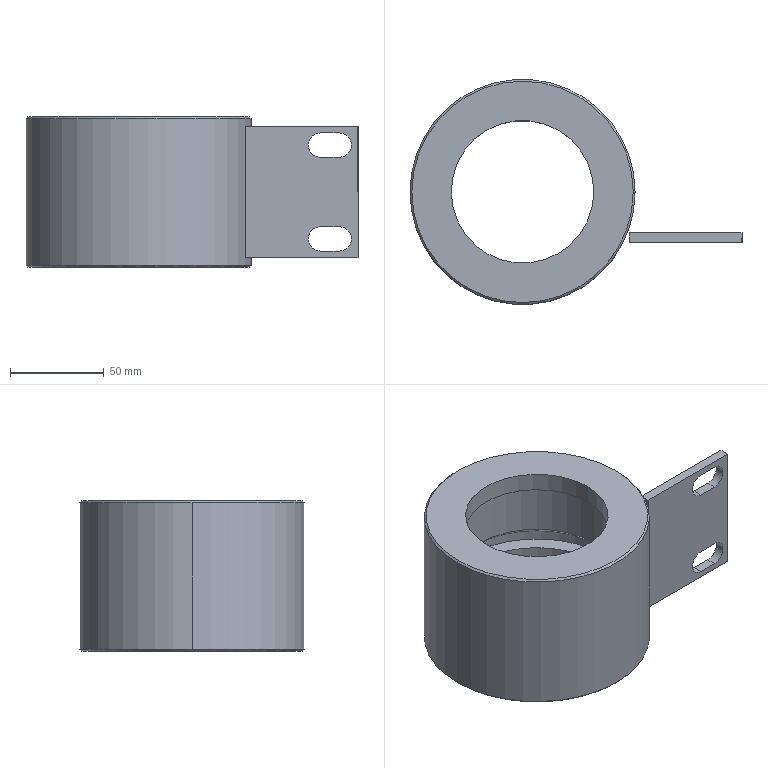Part | SolidWorks | features ICE 5, Chamfer 3, Cut 1, Extrusion 1 | 2 solids | 45 faces | box 177 x 120 x 80 mm | volume 437085 mm3 | cylinder 20 | plane 17 | cone 8 | commonest cylinder face diameters 13 x6 85 x6 76 x2 100 x2 101 x2 120 x2
STEP:
#1=CARTESIAN_POINT('',(42.5,0.,41.));
#2=VERTEX_POINT('',#1);
#3=CARTESIAN_POINT('',(-42.5,0.,41.));
#4=VERTEX_POINT('',#3);
#5=CARTESIAN_POINT('',(0.,0.,41.));
#6=DIRECTION('',(0.,0.,-1.));
#7=DIRECTION('',(-1.,0.,0.));
#8=AXIS2_PLACEMENT_3D('',#5,#6,#7);
#9=CIRCLE('',#8,42.5);
#10=EDGE_CURVE('',#2,#4,#9,.T.);
#11=ORIENTED_EDGE('',*,*,#10,.F.);
#12=CARTESIAN_POINT('',(45.5,0.,38.));
#13=VERTEX_POINT('',#12);
#14=CARTESIAN_POINT('',(42.5,0.,41.));
#15=DIRECTION('',(0.7071,0.,-0.7071));
#16=VECTOR('',#15,1000.);
#17=LINE('',#14,#16);
#18=EDGE_CURVE('',#2,#13,#17,.T.);
#19=ORIENTED_EDGE('',*,*,#18,.T.);
#20=CARTESIAN_POINT('',(-45.5,0.,38.));
#21=VERTEX_POINT('',#20);
#22=CARTESIAN_POINT('',(0.,0.,38.));
#23=DIRECTION('',(0.,0.,1.));
#24=DIRECTION('',(-1.,0.,0.));
#25=AXIS2_PLACEMENT_3D('',#22,#23,#24);
#26=CIRCLE('',#25,45.5);
#27=EDGE_CURVE('',#21,#13,#26,.T.);
#28=ORIENTED_EDGE('',*,*,#27,.F.);
#29=CARTESIAN_POINT('',(-42.5,0.,41.));
#30=DIRECTION('',(-0.7071,0.,-0.7071));
#31=VECTOR('',#30,1000.);
#32=LINE('',#29,#31);
#33=EDGE_CURVE('',#4,#21,#32,.T.);
#34=ORIENTED_EDGE('',*,*,#33,.F.);
#35=EDGE_LOOP('',(#11,#19,#28,#34));
#36=FACE_OUTER_BOUND('',#35,.T.);
#37=CARTESIAN_POINT('',(0.,0.,41.));
#38=DIRECTION('',(0.,0.,-1.));
#39=DIRECTION('',(-1.,0.,0.));
#40=AXIS2_PLACEMENT_3D('',#37,#38,#39);
#41=CONICAL_SURFACE('',#40,42.5,0.7854);
#42=ADVANCED_FACE('',(#36),#41,.F.);
#43=CARTESIAN_POINT('',(50.5,0.,38.));
#44=VERTEX_POINT('',#43);
#45=CARTESIAN_POINT('',(-50.5,0.,38.));
#46=VERTEX_POINT('',#45);
#47=CARTESIAN_POINT('',(0.,0.,38.));
#48=DIRECTION('',(0.,0.,-1.));
#49=DIRECTION('',(-1.,0.,0.));
#50=AXIS2_PLACEMENT_3D('',#47,#48,#49);
#51=CIRCLE('',#50,50.5);
#52=EDGE_CURVE('',#44,#46,#51,.T.);
#53=ORIENTED_EDGE('',*,*,#52,.F.);
#54=CARTESIAN_POINT('',(50.5,0.,29.));
#55=VERTEX_POINT('',#54);
#56=CARTESIAN_POINT('',(50.5,0.,38.));
#57=DIRECTION('',(0.,0.,-1.));
#58=VECTOR('',#57,1000.);
#59=LINE('',#56,#58);
#60=EDGE_CURVE('',#44,#55,#59,.T.);
#61=ORIENTED_EDGE('',*,*,#60,.T.);
#62=CARTESIAN_POINT('',(-50.5,0.,29.));
#63=VERTEX_POINT('',#62);
#64=CARTESIAN_POINT('',(0.,0.,29.));
#65=DIRECTION('',(0.,0.,-1.));
#66=DIRECTION('',(-1.,0.,0.));
#67=AXIS2_PLACEMENT_3D('',#64,#65,#66);
#68=CIRCLE('',#67,50.5);
#69=EDGE_CURVE('',#55,#63,#68,.T.);
#70=ORIENTED_EDGE('',*,*,#69,.T.);
#71=CARTESIAN_POINT('',(-50.5,0.,38.));
#72=DIRECTION('',(0.,0.,-1.));
#73=VECTOR('',#72,1000.);
#74=LINE('',#71,#73);
#75=EDGE_CURVE('',#46,#63,#74,.T.);
#76=ORIENTED_EDGE('',*,*,#75,.F.);
#77=EDGE_LOOP('',(#53,#61,#70,#76));
#78=FACE_OUTER_BOUND('',#77,.T.);
#79=CARTESIAN_POINT('',(0.,0.,38.));
#80=DIRECTION('',(0.,0.,-1.));
#81=DIRECTION('',(-1.,0.,0.));
#82=AXIS2_PLACEMENT_3D('',#79,#80,#81);
#83=CYLINDRICAL_SURFACE('',#82,50.5);
#84=ADVANCED_FACE('',(#78),#83,.F.);
#85=CARTESIAN_POINT('',(42.5,0.,22.));
#86=VERTEX_POINT('',#85);
#87=CARTESIAN_POINT('',(-42.5,0.,22.));
#88=VERTEX_POINT('',#87);
#89=CARTESIAN_POINT('',(0.,0.,22.));
#90=DIRECTION('',(0.,0.,-1.));
#91=DIRECTION('',(-1.,0.,0.));
#92=AXIS2_PLACEMENT_3D('',#89,#90,#91);
#93=CIRCLE('',#92,42.5);
#94=EDGE_CURVE('',#86,#88,#93,.T.);
#95=ORIENTED_EDGE('',*,*,#94,.F.);
#96=CARTESIAN_POINT('',(45.5,0.,19.));
#97=VERTEX_POINT('',#96);
#98=CARTESIAN_POINT('',(42.5,0.,22.));
#99=DIRECTION('',(0.7071,0.,-0.7071));
#100=VECTOR('',#99,1000.);
#101=LINE('',#98,#100);
#102=EDGE_CURVE('',#86,#97,#101,.T.);
#103=ORIENTED_EDGE('',*,*,#102,.T.);
#104=CARTESIAN_POINT('',(-45.5,0.,19.));
#105=VERTEX_POINT('',#104);
#106=CARTESIAN_POINT('',(0.,0.,19.));
#107=DIRECTION('',(0.,0.,1.));
#108=DIRECTION('',(-1.,0.,0.));
#109=AXIS2_PLACEMENT_3D('',#106,#107,#108);
#110=CIRCLE('',#109,45.5);
#111=EDGE_CURVE('',#105,#97,#110,.T.);
#112=ORIENTED_EDGE('',*,*,#111,.F.);
#113=CARTESIAN_POINT('',(-42.5,0.,22.));
#114=DIRECTION('',(-0.7071,0.,-0.7071));
#115=VECTOR('',#114,1000.);
#116=LINE('',#113,#115);
#117=EDGE_CURVE('',#88,#105,#116,.T.);
#118=ORIENTED_EDGE('',*,*,#117,.F.);
#119=EDGE_LOOP('',(#95,#103,#112,#118));
#120=FACE_OUTER_BOUND('',#119,.T.);
#121=CARTESIAN_POINT('',(0.,0.,22.));
#122=DIRECTION('',(0.,0.,-1.));
#123=DIRECTION('',(-1.,0.,0.));
#124=AXIS2_PLACEMENT_3D('',#121,#122,#123);
#125=CONICAL_SURFACE('',#124,42.5,0.7854);
#126=ADVANCED_FACE('',(#120),#125,.F.);
#127=CARTESIAN_POINT('',(50.,0.,19.));
#128=VERTEX_POINT('',#127);
#129=CARTESIAN_POINT('',(-50.,0.,19.));
#130=VERTEX_POINT('',#129);
#131=CARTESIAN_POINT('',(0.,0.,19.));
#132=DIRECTION('',(0.,0.,-1.));
#133=DIRECTION('',(-1.,0.,0.));
#134=AXIS2_PLACEMENT_3D('',#131,#132,#133);
#135=CIRCLE('',#134,50.);
#136=EDGE_CURVE('',#128,#130,#135,.T.);
#137=ORIENTED_EDGE('',*,*,#136,.F.);
#138=CARTESIAN_POINT('',(50.,0.,10.));
#139=VERTEX_POINT('',#138);
#140=CARTESIAN_POINT('',(50.,0.,19.));
#141=DIRECTION('',(0.,0.,-1.));
#142=VECTOR('',#141,1000.);
#143=LINE('',#140,#142);
#144=EDGE_CURVE('',#128,#139,#143,.T.);
#145=ORIENTED_EDGE('',*,*,#144,.T.);
#146=CARTESIAN_POINT('',(-50.,0.,10.));
#147=VERTEX_POINT('',#146);
#148=CARTESIAN_POINT('',(0.,0.,10.));
#149=DIRECTION('',(0.,0.,-1.));
#150=DIRECTION('',(-1.,0.,0.));
#151=AXIS2_PLACEMENT_3D('',#148,#149,#150);
#152=CIRCLE('',#151,50.);
#153=EDGE_CURVE('',#139,#147,#152,.T.);
#154=ORIENTED_EDGE('',*,*,#153,.T.);
#155=CARTESIAN_POINT('',(-50.,0.,19.));
#156=DIRECTION('',(0.,0.,-1.));
#157=VECTOR('',#156,1000.);
#158=LINE('',#155,#157);
#159=EDGE_CURVE('',#130,#147,#158,.T.);
#160=ORIENTED_EDGE('',*,*,#159,.F.);
#161=EDGE_LOOP('',(#137,#145,#154,#160));
#162=FACE_OUTER_BOUND('',#161,.T.);
#163=CARTESIAN_POINT('',(0.,0.,19.));
#164=DIRECTION('',(0.,0.,-1.));
#165=DIRECTION('',(-1.,0.,0.));
#166=AXIS2_PLACEMENT_3D('',#163,#164,#165);
#167=CYLINDRICAL_SURFACE('',#166,50.);
#168=ADVANCED_FACE('',(#162),#167,.F.);
#169=CARTESIAN_POINT('',(59.,0.,80.));
#170=VERTEX_POINT('',#169);
#171=CARTESIAN_POINT('',(-59.,0.,80.));
#172=VERTEX_POINT('',#171);
#173=CARTESIAN_POINT('',(0.,0.,80.));
#174=DIRECTION('',(0.,0.,1.));
#175=DIRECTION('',(1.,0.,0.));
#176=AXIS2_PLACEMENT_3D('',#173,#174,#175);
#177=CIRCLE('',#176,59.);
#178=EDGE_CURVE('',#170,#172,#177,.T.);
#179=ORIENTED_EDGE('',*,*,#178,.F.);
#180=CARTESIAN_POINT('',(60.,0.,79.));
#181=VERTEX_POINT('',#180);
#182=CARTESIAN_POINT('',(59.,0.,80.));
#183=DIRECTION('',(0.7071,0.,-0.7071));
#184=VECTOR('',#183,1000.);
#185=LINE('',#182,#184);
#186=EDGE_CURVE('',#170,#181,#185,.T.);
#187=ORIENTED_EDGE('',*,*,#186,.T.);
#188=CARTESIAN_POINT('',(-60.,0.,79.));
#189=VERTEX_POINT('',#188);
#190=CARTESIAN_POINT('',(0.,0.,79.));
#191=DIRECTION('',(0.,0.,-1.));
#192=DIRECTION('',(1.,0.,0.));
#193=AXIS2_PLACEMENT_3D('',#190,#191,#192);
#194=CIRCLE('',#193,60.);
#195=EDGE_CURVE('',#189,#181,#194,.T.);
#196=ORIENTED_EDGE('',*,*,#195,.F.);
#197=CARTESIAN_POINT('',(-59.,0.,80.));
#198=DIRECTION('',(-0.7071,0.,-0.7071));
#199=VECTOR('',#198,1000.);
#200=LINE('',#197,#199);
#201=EDGE_CURVE('',#172,#189,#200,.T.);
#202=ORIENTED_EDGE('',*,*,#201,.F.);
#203=EDGE_LOOP('',(#179,#187,#196,#202));
#204=FACE_OUTER_BOUND('',#203,.T.);
#205=CARTESIAN_POINT('',(0.,0.,80.));
#206=DIRECTION('',(0.,0.,-1.));
#207=DIRECTION('',(-1.,0.,0.));
#208=AXIS2_PLACEMENT_3D('',#205,#206,#207);
#209=CONICAL_SURFACE('',#208,59.,0.7854);
#210=ADVANCED_FACE('',(#204),#209,.T.);
#211=CARTESIAN_POINT('',(-59.,0.,0.));
#212=VERTEX_POINT('',#211);
#213=CARTESIAN_POINT('',(59.,0.,0.));
#214=VERTEX_POINT('',#213);
#215=CARTESIAN_POINT('',(0.,0.,0.));
#216=DIRECTION('',(0.,0.,-1.));
#217=DIRECTION('',(1.,0.,0.));
#218=AXIS2_PLACEMENT_3D('',#215,#216,#217);
#219=CIRCLE('',#218,59.);
#220=EDGE_CURVE('',#212,#214,#219,.T.);
#221=ORIENTED_EDGE('',*,*,#220,.F.);
#222=CARTESIAN_POINT('',(-60.,0.,1.));
#223=VERTEX_POINT('',#222);
#224=CARTESIAN_POINT('',(-60.,0.,1.));
#225=DIRECTION('',(-0.7071,0.,0.7071));
#226=VECTOR('',#225,1000.);
#227=LINE('',#224,#226);
#228=EDGE_CURVE('',#212,#223,#227,.T.);
#229=ORIENTED_EDGE('',*,*,#228,.T.);
#230=CARTESIAN_POINT('',(60.,0.,1.));
#231=VERTEX_POINT('',#230);
#232=CARTESIAN_POINT('',(0.,0.,1.));
#233=DIRECTION('',(0.,0.,1.));
#234=DIRECTION('',(1.,0.,0.));
#235=AXIS2_PLACEMENT_3D('',#232,#233,#234);
#236=CIRCLE('',#235,60.);
#237=EDGE_CURVE('',#231,#223,#236,.T.);
#238=ORIENTED_EDGE('',*,*,#237,.F.);
#239=CARTESIAN_POINT('',(60.,0.,1.));
#240=DIRECTION('',(0.7071,0.,0.7071));
#241=VECTOR('',#240,1000.);
#242=LINE('',#239,#241);
#243=EDGE_CURVE('',#214,#231,#242,.T.);
#244=ORIENTED_EDGE('',*,*,#243,.F.);
#245=EDGE_LOOP('',(#221,#229,#238,#244));
#246=FACE_OUTER_BOUND('',#245,.T.);
#247=CARTESIAN_POINT('',(0.,0.,1.));
#248=DIRECTION('',(0.,0.,1.));
#249=DIRECTION('',(1.,0.,0.));
#250=AXIS2_PLACEMENT_3D('',#247,#248,#249);
#251=CONICAL_SURFACE('',#250,60.,0.7854);
#252=ADVANCED_FACE('',(#246),#251,.T.);
#253=CARTESIAN_POINT('',(38.,0.,70.));
#254=VERTEX_POINT('',#253);
#255=CARTESIAN_POINT('',(-38.,0.,70.));
#256=VERTEX_POINT('',#255);
#257=CARTESIAN_POINT('',(0.,0.,70.));
#258=DIRECTION('',(0.,0.,-1.));
#259=DIRECTION('',(-1.,0.,0.));
#260=AXIS2_PLACEMENT_3D('',#257,#258,#259);
#261=CIRCLE('',#260,38.);
#262=EDGE_CURVE('',#254,#256,#261,.T.);
#263=ORIENTED_EDGE('',*,*,#262,.T.);
#264=CARTESIAN_POINT('',(-38.,0.,80.));
#265=VERTEX_POINT('',#264);
#266=CARTESIAN_POINT('',(-38.,0.,10.));
#267=DIRECTION('',(0.,0.,1.));
#268=VECTOR('',#267,1000.);
#269=LINE('',#266,#268);
#270=EDGE_CURVE('',#256,#265,#269,.T.);
#271=ORIENTED_EDGE('',*,*,#270,.T.);
#272=CARTESIAN_POINT('',(38.,0.,80.));
#273=VERTEX_POINT('',#272);
#274=CARTESIAN_POINT('',(0.,0.,80.));
#275=DIRECTION('',(0.,0.,1.));
#276=DIRECTION('',(1.,0.,0.));
#277=AXIS2_PLACEMENT_3D('',#274,#275,#276);
#278=CIRCLE('',#277,38.);
#279=EDGE_CURVE('',#265,#273,#278,.T.);
#280=ORIENTED_EDGE('',*,*,#279,.T.);
#281=CARTESIAN_POINT('',(38.,0.,10.));
#282=DIRECTION('',(0.,0.,1.));
#283=VECTOR('',#282,1000.);
#284=LINE('',#281,#283);
#285=EDGE_CURVE('',#254,#273,#284,.T.);
#286=ORIENTED_EDGE('',*,*,#285,.F.);
#287=EDGE_LOOP('',(#263,#271,#280,#286));
#288=FACE_OUTER_BOUND('',#287,.T.);
#289=CARTESIAN_POINT('',(0.,0.,10.));
#290=DIRECTION('',(0.,0.,1.));
#291=DIRECTION('',(1.,0.,0.));
#292=AXIS2_PLACEMENT_3D('',#289,#290,#291);
#293=CYLINDRICAL_SURFACE('',#292,38.);
#294=ADVANCED_FACE('',(#288),#293,.F.);
#295=CARTESIAN_POINT('',(42.5,0.,10.));
#296=VERTEX_POINT('',#295);
#297=CARTESIAN_POINT('',(-42.5,0.,10.));
#298=VERTEX_POINT('',#297);
#299=CARTESIAN_POINT('',(0.,0.,10.));
#300=DIRECTION('',(0.,0.,-1.));
#301=DIRECTION('',(-1.,0.,0.));
#302=AXIS2_PLACEMENT_3D('',#299,#300,#301);
#303=CIRCLE('',#302,42.5);
#304=EDGE_CURVE('',#296,#298,#303,.T.);
#305=ORIENTED_EDGE('',*,*,#304,.F.);
#306=CARTESIAN_POINT('',(42.5,0.,0.));
#307=VERTEX_POINT('',#306);
#308=CARTESIAN_POINT('',(42.5,0.,70.));
#309=DIRECTION('',(0.,0.,-1.));
#310=VECTOR('',#309,1000.);
#311=LINE('',#308,#310);
#312=EDGE_CURVE('',#296,#307,#311,.T.);
#313=ORIENTED_EDGE('',*,*,#312,.T.);
#314=CARTESIAN_POINT('',(-42.5,0.,0.));
#315=VERTEX_POINT('',#314);
#316=CARTESIAN_POINT('',(0.,0.,0.));
#317=DIRECTION('',(0.,0.,-1.));
#318=DIRECTION('',(-1.,0.,0.));
#319=AXIS2_PLACEMENT_3D('',#316,#317,#318);
#320=CIRCLE('',#319,42.5);
#321=EDGE_CURVE('',#307,#315,#320,.T.);
#322=ORIENTED_EDGE('',*,*,#321,.T.);
#323=CARTESIAN_POINT('',(-42.5,0.,70.));
#324=DIRECTION('',(0.,0.,-1.));
#325=VECTOR('',#324,1000.);
#326=LINE('',#323,#325);
#327=EDGE_CURVE('',#298,#315,#326,.T.);
#328=ORIENTED_EDGE('',*,*,#327,.F.);
#329=EDGE_LOOP('',(#305,#313,#322,#328));
#330=FACE_OUTER_BOUND('',#329,.T.);
#331=CARTESIAN_POINT('',(0.,0.,70.));
#332=DIRECTION('',(0.,0.,-1.));
#333=DIRECTION('',(-1.,0.,0.));
#334=AXIS2_PLACEMENT_3D('',#331,#332,#333);
#335=CYLINDRICAL_SURFACE('',#334,42.5);
#336=ADVANCED_FACE('',(#330),#335,.F.);
#337=ORIENTED_EDGE('',*,*,#195,.T.);
#338=CARTESIAN_POINT('',(60.,0.,80.));
#339=DIRECTION('',(0.,0.,-1.));
#340=VECTOR('',#339,1000.);
#341=LINE('',#338,#340);
#342=EDGE_CURVE('',#181,#231,#341,.T.);
#343=ORIENTED_EDGE('',*,*,#342,.T.);
#344=ORIENTED_EDGE('',*,*,#237,.T.);
#345=CARTESIAN_POINT('',(-60.,0.,80.));
#346=DIRECTION('',(0.,0.,-1.));
#347=VECTOR('',#346,1000.);
#348=LINE('',#345,#347);
#349=EDGE_CURVE('',#189,#223,#348,.T.);
#350=ORIENTED_EDGE('',*,*,#349,.F.);
#351=EDGE_LOOP('',(#337,#343,#344,#350));
#352=FACE_OUTER_BOUND('',#351,.T.);
#353=CARTESIAN_POINT('',(0.,0.,80.));
#354=DIRECTION('',(0.,0.,-1.));
#355=DIRECTION('',(-1.,0.,0.));
#356=AXIS2_PLACEMENT_3D('',#353,#354,#355);
#357=CYLINDRICAL_SURFACE('',#356,60.);
#358=ADVANCED_FACE('',(#352),#357,.T.);
#359=CARTESIAN_POINT('',(42.5,0.,29.));
#360=VERTEX_POINT('',#359);
#361=CARTESIAN_POINT('',(-42.5,0.,29.));
#362=VERTEX_POINT('',#361);
#363=CARTESIAN_POINT('',(0.,0.,29.));
#364=DIRECTION('',(0.,0.,-1.));
#365=DIRECTION('',(-1.,0.,0.));
#366=AXIS2_PLACEMENT_3D('',#363,#364,#365);
#367=CIRCLE('',#366,42.5);
#368=EDGE_CURVE('',#360,#362,#367,.T.);
#369=ORIENTED_EDGE('',*,*,#368,.F.);
#370=CARTESIAN_POINT('',(42.5,0.,70.));
#371=DIRECTION('',(0.,0.,-1.));
#372=VECTOR('',#371,1000.);
#373=LINE('',#370,#372);
#374=EDGE_CURVE('',#360,#86,#373,.T.);
#375=ORIENTED_EDGE('',*,*,#374,.T.);
#376=ORIENTED_EDGE('',*,*,#94,.T.);
#377=CARTESIAN_POINT('',(-42.5,0.,70.));
#378=DIRECTION('',(0.,0.,-1.));
#379=VECTOR('',#378,1000.);
#380=LINE('',#377,#379);
#381=EDGE_CURVE('',#362,#88,#380,.T.);
#382=ORIENTED_EDGE('',*,*,#381,.F.);
#383=EDGE_LOOP('',(#369,#375,#376,#382));
#384=FACE_OUTER_BOUND('',#383,.T.);
#385=CARTESIAN_POINT('',(0.,0.,70.));
#386=DIRECTION('',(0.,0.,-1.));
#387=DIRECTION('',(-1.,0.,0.));
#388=AXIS2_PLACEMENT_3D('',#385,#386,#387);
#389=CYLINDRICAL_SURFACE('',#388,42.5);
#390=ADVANCED_FACE('',(#384),#389,.F.);
#391=CARTESIAN_POINT('',(42.5,0.,70.));
#392=VERTEX_POINT('',#391);
#393=CARTESIAN_POINT('',(-42.5,0.,70.));
#394=VERTEX_POINT('',#393);
#395=CARTESIAN_POINT('',(0.,0.,70.));
#396=DIRECTION('',(0.,0.,-1.));
#397=DIRECTION('',(-1.,0.,0.));
#398=AXIS2_PLACEMENT_3D('',#395,#396,#397);
#399=CIRCLE('',#398,42.5);
#400=EDGE_CURVE('',#392,#394,#399,.T.);
#401=ORIENTED_EDGE('',*,*,#400,.F.);
#402=CARTESIAN_POINT('',(42.5,0.,70.));
#403=DIRECTION('',(0.,0.,-1.));
#404=VECTOR('',#403,1000.);
#405=LINE('',#402,#404);
#406=EDGE_CURVE('',#392,#2,#405,.T.);
#407=ORIENTED_EDGE('',*,*,#406,.T.);
#408=ORIENTED_EDGE('',*,*,#10,.T.);
#409=CARTESIAN_POINT('',(-42.5,0.,70.));
#410=DIRECTION('',(0.,0.,-1.));
#411=VECTOR('',#410,1000.);
#412=LINE('',#409,#411);
#413=EDGE_CURVE('',#394,#4,#412,.T.);
#414=ORIENTED_EDGE('',*,*,#413,.F.);
#415=EDGE_LOOP('',(#401,#407,#408,#414));
#416=FACE_OUTER_BOUND('',#415,.T.);
#417=CARTESIAN_POINT('',(0.,0.,70.));
#418=DIRECTION('',(0.,0.,-1.));
#419=DIRECTION('',(-1.,0.,0.));
#420=AXIS2_PLACEMENT_3D('',#417,#418,#419);
#421=CYLINDRICAL_SURFACE('',#420,42.5);
#422=ADVANCED_FACE('',(#416),#421,.F.);
#423=ORIENTED_EDGE('',*,*,#406,.F.);
#424=CARTESIAN_POINT('',(0.,0.,70.));
#425=DIRECTION('',(0.,0.,-1.));
#426=DIRECTION('',(-1.,0.,0.));
#427=AXIS2_PLACEMENT_3D('',#424,#425,#426);
#428=CIRCLE('',#427,42.5);
#429=EDGE_CURVE('',#394,#392,#428,.T.);
#430=ORIENTED_EDGE('',*,*,#429,.F.);
#431=ORIENTED_EDGE('',*,*,#413,.T.);
#432=CARTESIAN_POINT('',(0.,0.,41.));
#433=DIRECTION('',(0.,0.,-1.));
#434=DIRECTION('',(-1.,0.,0.));
#435=AXIS2_PLACEMENT_3D('',#432,#433,#434);
#436=CIRCLE('',#435,42.5);
#437=EDGE_CURVE('',#4,#2,#436,.T.);
#438=ORIENTED_EDGE('',*,*,#437,.T.);
#439=EDGE_LOOP('',(#423,#430,#431,#438));
#440=FACE_OUTER_BOUND('',#439,.T.);
#441=CARTESIAN_POINT('',(0.,0.,70.));
#442=DIRECTION('',(0.,0.,-1.));
#443=DIRECTION('',(-1.,0.,0.));
#444=AXIS2_PLACEMENT_3D('',#441,#442,#443);
#445=CYLINDRICAL_SURFACE('',#444,42.5);
#446=ADVANCED_FACE('',(#440),#445,.F.);
#447=ORIENTED_EDGE('',*,*,#374,.F.);
#448=CARTESIAN_POINT('',(0.,0.,29.));
#449=DIRECTION('',(0.,0.,-1.));
#450=DIRECTION('',(-1.,0.,0.));
#451=AXIS2_PLACEMENT_3D('',#448,#449,#450);
#452=CIRCLE('',#451,42.5);
#453=EDGE_CURVE('',#362,#360,#452,.T.);
#454=ORIENTED_EDGE('',*,*,#453,.F.);
#455=ORIENTED_EDGE('',*,*,#381,.T.);
#456=CARTESIAN_POINT('',(0.,0.,22.));
#457=DIRECTION('',(0.,0.,-1.));
#458=DIRECTION('',(-1.,0.,0.));
#459=AXIS2_PLACEMENT_3D('',#456,#457,#458);
#460=CIRCLE('',#459,42.5);
#461=EDGE_CURVE('',#88,#86,#460,.T.);
#462=ORIENTED_EDGE('',*,*,#461,.T.);
#463=EDGE_LOOP('',(#447,#454,#455,#462));
#464=FACE_OUTER_BOUND('',#463,.T.);
#465=CARTESIAN_POINT('',(0.,0.,70.));
#466=DIRECTION('',(0.,0.,-1.));
#467=DIRECTION('',(-1.,0.,0.));
#468=AXIS2_PLACEMENT_3D('',#465,#466,#467);
#469=CYLINDRICAL_SURFACE('',#468,42.5);
#470=ADVANCED_FACE('',(#464),#469,.F.);
#471=ORIENTED_EDGE('',*,*,#342,.F.);
#472=CARTESIAN_POINT('',(0.,0.,79.));
#473=DIRECTION('',(0.,0.,-1.));
#474=DIRECTION('',(1.,0.,0.));
#475=AXIS2_PLACEMENT_3D('',#472,#473,#474);
#476=CIRCLE('',#475,60.);
#477=EDGE_CURVE('',#181,#189,#476,.T.);
#478=ORIENTED_EDGE('',*,*,#477,.T.);
#479=ORIENTED_EDGE('',*,*,#349,.T.);
#480=CARTESIAN_POINT('',(0.,0.,1.));
#481=DIRECTION('',(0.,0.,1.));
#482=DIRECTION('',(1.,0.,0.));
#483=AXIS2_PLACEMENT_3D('',#480,#481,#482);
#484=CIRCLE('',#483,60.);
#485=EDGE_CURVE('',#223,#231,#484,.T.);
#486=ORIENTED_EDGE('',*,*,#485,.T.);
#487=EDGE_LOOP('',(#471,#478,#479,#486));
#488=FACE_OUTER_BOUND('',#487,.T.);
#489=CARTESIAN_POINT('',(0.,0.,80.));
#490=DIRECTION('',(0.,0.,-1.));
#491=DIRECTION('',(-1.,0.,0.));
#492=AXIS2_PLACEMENT_3D('',#489,#490,#491);
#493=CYLINDRICAL_SURFACE('',#492,60.);
#494=ADVANCED_FACE('',(#488),#493,.T.);
#495=CARTESIAN_POINT('',(0.,0.,80.));
#496=DIRECTION('',(0.,0.,1.));
#497=DIRECTION('',(1.,0.,0.));
#498=AXIS2_PLACEMENT_3D('',#495,#496,#497);
#499=CIRCLE('',#498,59.);
#500=EDGE_CURVE('',#172,#170,#499,.T.);
#501=ORIENTED_EDGE('',*,*,#500,.T.);
#502=ORIENTED_EDGE('',*,*,#178,.T.);
#503=EDGE_LOOP('',(#501,#502));
#504=FACE_OUTER_BOUND('',#503,.T.);
#505=CARTESIAN_POINT('',(0.,0.,80.));
#506=DIRECTION('',(0.,0.,1.));
#507=DIRECTION('',(1.,0.,0.));
#508=AXIS2_PLACEMENT_3D('',#505,#506,#507);
#509=CIRCLE('',#508,38.);
#510=EDGE_CURVE('',#273,#265,#509,.T.);
#511=ORIENTED_EDGE('',*,*,#510,.F.);
#512=ORIENTED_EDGE('',*,*,#279,.F.);
#513=EDGE_LOOP('',(#511,#512));
#514=FACE_BOUND('',#513,.T.);
#515=CARTESIAN_POINT('',(0.,0.,80.));
#516=DIRECTION('',(0.,0.,1.));
#517=DIRECTION('',(1.,0.,0.));
#518=AXIS2_PLACEMENT_3D('',#515,#516,#517);
#519=PLANE('',#518);
#520=ADVANCED_FACE('',(#504,#514),#519,.T.);
#521=CARTESIAN_POINT('',(0.,0.,0.));
#522=DIRECTION('',(0.,0.,-1.));
#523=DIRECTION('',(1.,0.,0.));
#524=AXIS2_PLACEMENT_3D('',#521,#522,#523);
#525=CIRCLE('',#524,59.);
#526=EDGE_CURVE('',#214,#212,#525,.T.);
#527=ORIENTED_EDGE('',*,*,#526,.T.);
#528=ORIENTED_EDGE('',*,*,#220,.T.);
#529=EDGE_LOOP('',(#527,#528));
#530=FACE_OUTER_BOUND('',#529,.T.);
#531=CARTESIAN_POINT('',(0.,0.,0.));
#532=DIRECTION('',(0.,0.,-1.));
#533=DIRECTION('',(-1.,0.,0.));
#534=AXIS2_PLACEMENT_3D('',#531,#532,#533);
#535=CIRCLE('',#534,42.5);
#536=EDGE_CURVE('',#315,#307,#535,.T.);
#537=ORIENTED_EDGE('',*,*,#536,.F.);
#538=ORIENTED_EDGE('',*,*,#321,.F.);
#539=EDGE_LOOP('',(#537,#538));
#540=FACE_BOUND('',#539,.T.);
#541=CARTESIAN_POINT('',(0.,0.,0.));
#542=DIRECTION('',(0.,0.,1.));
#543=DIRECTION('',(1.,0.,0.));
#544=AXIS2_PLACEMENT_3D('',#541,#542,#543);
#545=PLANE('',#544);
#546=ADVANCED_FACE('',(#530,#540),#545,.F.);
#547=ORIENTED_EDGE('',*,*,#312,.F.);
#548=CARTESIAN_POINT('',(0.,0.,10.));
#549=DIRECTION('',(0.,0.,-1.));
#550=DIRECTION('',(-1.,0.,0.));
#551=AXIS2_PLACEMENT_3D('',#548,#549,#550);
#552=CIRCLE('',#551,42.5);
#553=EDGE_CURVE('',#298,#296,#552,.T.);
#554=ORIENTED_EDGE('',*,*,#553,.F.);
#555=ORIENTED_EDGE('',*,*,#327,.T.);
#556=ORIENTED_EDGE('',*,*,#536,.T.);
#557=EDGE_LOOP('',(#547,#554,#555,#556));
#558=FACE_OUTER_BOUND('',#557,.T.);
#559=CARTESIAN_POINT('',(0.,0.,70.));
#560=DIRECTION('',(0.,0.,-1.));
#561=DIRECTION('',(-1.,0.,0.));
#562=AXIS2_PLACEMENT_3D('',#559,#560,#561);
#563=CYLINDRICAL_SURFACE('',#562,42.5);
#564=ADVANCED_FACE('',(#558),#563,.F.);
#565=ORIENTED_EDGE('',*,*,#262,.F.);
#566=CARTESIAN_POINT('',(0.,0.,70.));
#567=DIRECTION('',(0.,0.,-1.));
#568=DIRECTION('',(-1.,0.,0.));
#569=AXIS2_PLACEMENT_3D('',#566,#567,#568);
#570=CIRCLE('',#569,38.);
#571=EDGE_CURVE('',#256,#254,#570,.T.);
#572=ORIENTED_EDGE('',*,*,#571,.F.);
#573=EDGE_LOOP('',(#565,#572));
#574=FACE_BOUND('',#573,.T.);
#575=ORIENTED_EDGE('',*,*,#429,.T.);
#576=ORIENTED_EDGE('',*,*,#400,.T.);
#577=EDGE_LOOP('',(#575,#576));
#578=FACE_OUTER_BOUND('',#577,.T.);
#579=CARTESIAN_POINT('',(0.,0.,70.));
#580=DIRECTION('',(0.,0.,-1.));
#581=DIRECTION('',(-1.,0.,0.));
#582=AXIS2_PLACEMENT_3D('',#579,#580,#581);
#583=PLANE('',#582);
#584=ADVANCED_FACE('',(#574,#578),#583,.T.);
#585=ORIENTED_EDGE('',*,*,#270,.F.);
#586=ORIENTED_EDGE('',*,*,#571,.T.);
#587=ORIENTED_EDGE('',*,*,#285,.T.);
#588=ORIENTED_EDGE('',*,*,#510,.T.);
#589=EDGE_LOOP('',(#585,#586,#587,#588));
#590=FACE_OUTER_BOUND('',#589,.T.);
#591=CARTESIAN_POINT('',(0.,0.,10.));
#592=DIRECTION('',(0.,0.,1.));
#593=DIRECTION('',(1.,0.,0.));
#594=AXIS2_PLACEMENT_3D('',#591,#592,#593);
#595=CYLINDRICAL_SURFACE('',#594,38.);
#596=ADVANCED_FACE('',(#590),#595,.F.);
#597=ORIENTED_EDGE('',*,*,#228,.F.);
#598=ORIENTED_EDGE('',*,*,#526,.F.);
#599=ORIENTED_EDGE('',*,*,#243,.T.);
#600=ORIENTED_EDGE('',*,*,#485,.F.);
#601=EDGE_LOOP('',(#597,#598,#599,#600));
#602=FACE_OUTER_BOUND('',#601,.T.);
#603=CARTESIAN_POINT('',(0.,0.,1.));
#604=DIRECTION('',(0.,0.,1.));
#605=DIRECTION('',(1.,0.,0.));
#606=AXIS2_PLACEMENT_3D('',#603,#604,#605);
#607=CONICAL_SURFACE('',#606,60.,0.7854);
#608=ADVANCED_FACE('',(#602),#607,.T.);
#609=ORIENTED_EDGE('',*,*,#186,.F.);
#610=ORIENTED_EDGE('',*,*,#500,.F.);
#611=ORIENTED_EDGE('',*,*,#201,.T.);
#612=ORIENTED_EDGE('',*,*,#477,.F.);
#613=EDGE_LOOP('',(#609,#610,#611,#612));
#614=FACE_OUTER_BOUND('',#613,.T.);
#615=CARTESIAN_POINT('',(0.,0.,80.));
#616=DIRECTION('',(0.,0.,-1.));
#617=DIRECTION('',(-1.,0.,0.));
#618=AXIS2_PLACEMENT_3D('',#615,#616,#617);
#619=CONICAL_SURFACE('',#618,59.,0.7854);
#620=ADVANCED_FACE('',(#614),#619,.T.);
#621=ORIENTED_EDGE('',*,*,#144,.F.);
#622=CARTESIAN_POINT('',(0.,0.,19.));
#623=DIRECTION('',(0.,0.,-1.));
#624=DIRECTION('',(-1.,0.,0.));
#625=AXIS2_PLACEMENT_3D('',#622,#623,#624);
#626=CIRCLE('',#625,50.);
#627=EDGE_CURVE('',#130,#128,#626,.T.);
#628=ORIENTED_EDGE('',*,*,#627,.F.);
#629=ORIENTED_EDGE('',*,*,#159,.T.);
#630=CARTESIAN_POINT('',(0.,0.,10.));
#631=DIRECTION('',(0.,0.,-1.));
#632=DIRECTION('',(-1.,0.,0.));
#633=AXIS2_PLACEMENT_3D('',#630,#631,#632);
#634=CIRCLE('',#633,50.);
#635=EDGE_CURVE('',#147,#139,#634,.T.);
#636=ORIENTED_EDGE('',*,*,#635,.T.);
#637=EDGE_LOOP('',(#621,#628,#629,#636));
#638=FACE_OUTER_BOUND('',#637,.T.);
#639=CARTESIAN_POINT('',(0.,0.,19.));
#640=DIRECTION('',(0.,0.,-1.));
#641=DIRECTION('',(-1.,0.,0.));
#642=AXIS2_PLACEMENT_3D('',#639,#640,#641);
#643=CYLINDRICAL_SURFACE('',#642,50.);
#644=ADVANCED_FACE('',(#638),#643,.F.);
#645=ORIENTED_EDGE('',*,*,#111,.T.);
#646=CARTESIAN_POINT('',(0.,0.,19.));
#647=DIRECTION('',(0.,0.,1.));
#648=DIRECTION('',(-1.,0.,0.));
#649=AXIS2_PLACEMENT_3D('',#646,#647,#648);
#650=CIRCLE('',#649,45.5);
#651=EDGE_CURVE('',#97,#105,#650,.T.);
#652=ORIENTED_EDGE('',*,*,#651,.T.);
#653=EDGE_LOOP('',(#645,#652));
#654=FACE_BOUND('',#653,.T.);
#655=ORIENTED_EDGE('',*,*,#627,.T.);
#656=ORIENTED_EDGE('',*,*,#136,.T.);
#657=EDGE_LOOP('',(#655,#656));
#658=FACE_OUTER_BOUND('',#657,.T.);
#659=CARTESIAN_POINT('',(0.,0.,19.));
#660=DIRECTION('',(0.,0.,-1.));
#661=DIRECTION('',(-1.,0.,0.));
#662=AXIS2_PLACEMENT_3D('',#659,#660,#661);
#663=PLANE('',#662);
#664=ADVANCED_FACE('',(#654,#658),#663,.T.);
#665=ORIENTED_EDGE('',*,*,#553,.T.);
#666=ORIENTED_EDGE('',*,*,#304,.T.);
#667=EDGE_LOOP('',(#665,#666));
#668=FACE_BOUND('',#667,.T.);
#669=ORIENTED_EDGE('',*,*,#635,.F.);
#670=ORIENTED_EDGE('',*,*,#153,.F.);
#671=EDGE_LOOP('',(#669,#670));
#672=FACE_OUTER_BOUND('',#671,.T.);
#673=CARTESIAN_POINT('',(0.,0.,10.));
#674=DIRECTION('',(0.,0.,-1.));
#675=DIRECTION('',(-1.,0.,0.));
#676=AXIS2_PLACEMENT_3D('',#673,#674,#675);
#677=PLANE('',#676);
#678=ADVANCED_FACE('',(#668,#672),#677,.F.);
#679=ORIENTED_EDGE('',*,*,#102,.F.);
#680=ORIENTED_EDGE('',*,*,#461,.F.);
#681=ORIENTED_EDGE('',*,*,#117,.T.);
#682=ORIENTED_EDGE('',*,*,#651,.F.);
#683=EDGE_LOOP('',(#679,#680,#681,#682));
#684=FACE_OUTER_BOUND('',#683,.T.);
#685=CARTESIAN_POINT('',(0.,0.,22.));
#686=DIRECTION('',(0.,0.,-1.));
#687=DIRECTION('',(-1.,0.,0.));
#688=AXIS2_PLACEMENT_3D('',#685,#686,#687);
#689=CONICAL_SURFACE('',#688,42.5,0.7854);
#690=ADVANCED_FACE('',(#684),#689,.F.);
#691=ORIENTED_EDGE('',*,*,#60,.F.);
#692=CARTESIAN_POINT('',(0.,0.,38.));
#693=DIRECTION('',(0.,0.,-1.));
#694=DIRECTION('',(-1.,0.,0.));
#695=AXIS2_PLACEMENT_3D('',#692,#693,#694);
#696=CIRCLE('',#695,50.5);
#697=EDGE_CURVE('',#46,#44,#696,.T.);
#698=ORIENTED_EDGE('',*,*,#697,.F.);
#699=ORIENTED_EDGE('',*,*,#75,.T.);
#700=CARTESIAN_POINT('',(0.,0.,29.));
#701=DIRECTION('',(0.,0.,-1.));
#702=DIRECTION('',(-1.,0.,0.));
#703=AXIS2_PLACEMENT_3D('',#700,#701,#702);
#704=CIRCLE('',#703,50.5);
#705=EDGE_CURVE('',#63,#55,#704,.T.);
#706=ORIENTED_EDGE('',*,*,#705,.T.);
#707=EDGE_LOOP('',(#691,#698,#699,#706));
#708=FACE_OUTER_BOUND('',#707,.T.);
#709=CARTESIAN_POINT('',(0.,0.,38.));
#710=DIRECTION('',(0.,0.,-1.));
#711=DIRECTION('',(-1.,0.,0.));
#712=AXIS2_PLACEMENT_3D('',#709,#710,#711);
#713=CYLINDRICAL_SURFACE('',#712,50.5);
#714=ADVANCED_FACE('',(#708),#713,.F.);
#715=ORIENTED_EDGE('',*,*,#27,.T.);
#716=CARTESIAN_POINT('',(0.,0.,38.));
#717=DIRECTION('',(0.,0.,1.));
#718=DIRECTION('',(-1.,0.,0.));
#719=AXIS2_PLACEMENT_3D('',#716,#717,#718);
#720=CIRCLE('',#719,45.5);
#721=EDGE_CURVE('',#13,#21,#720,.T.);
#722=ORIENTED_EDGE('',*,*,#721,.T.);
#723=EDGE_LOOP('',(#715,#722));
#724=FACE_BOUND('',#723,.T.);
#725=ORIENTED_EDGE('',*,*,#697,.T.);
#726=ORIENTED_EDGE('',*,*,#52,.T.);
#727=EDGE_LOOP('',(#725,#726));
#728=FACE_OUTER_BOUND('',#727,.T.);
#729=CARTESIAN_POINT('',(0.,0.,38.));
#730=DIRECTION('',(0.,0.,-1.));
#731=DIRECTION('',(-1.,0.,0.));
#732=AXIS2_PLACEMENT_3D('',#729,#730,#731);
#733=PLANE('',#732);
#734=ADVANCED_FACE('',(#724,#728),#733,.T.);
#735=ORIENTED_EDGE('',*,*,#453,.T.);
#736=ORIENTED_EDGE('',*,*,#368,.T.);
#737=EDGE_LOOP('',(#735,#736));
#738=FACE_BOUND('',#737,.T.);
#739=ORIENTED_EDGE('',*,*,#705,.F.);
#740=ORIENTED_EDGE('',*,*,#69,.F.);
#741=EDGE_LOOP('',(#739,#740));
#742=FACE_OUTER_BOUND('',#741,.T.);
#743=CARTESIAN_POINT('',(0.,0.,29.));
#744=DIRECTION('',(0.,0.,-1.));
#745=DIRECTION('',(-1.,0.,0.));
#746=AXIS2_PLACEMENT_3D('',#743,#744,#745);
#747=PLANE('',#746);
#748=ADVANCED_FACE('',(#738,#742),#747,.F.);
#749=ORIENTED_EDGE('',*,*,#18,.F.);
#750=ORIENTED_EDGE('',*,*,#437,.F.);
#751=ORIENTED_EDGE('',*,*,#33,.T.);
#752=ORIENTED_EDGE('',*,*,#721,.F.);
#753=EDGE_LOOP('',(#749,#750,#751,#752));
#754=FACE_OUTER_BOUND('',#753,.T.);
#755=CARTESIAN_POINT('',(0.,0.,41.));
#756=DIRECTION('',(0.,0.,-1.));
#757=DIRECTION('',(-1.,0.,0.));
#758=AXIS2_PLACEMENT_3D('',#755,#756,#757);
#759=CONICAL_SURFACE('',#758,42.5,0.7854);
#760=ADVANCED_FACE('',(#754),#759,.F.);
#761=CLOSED_SHELL('',(#42,#84,#126,#168,#210,#252,#294,#336,#358,#390,#422,#446,#470,#494,#520,#546,#564,#584,#596,#608,#620,#644,#664,#678,#690,#714,#734,#748,#760));
#762=MANIFOLD_SOLID_BREP('',#761);
#763=CARTESIAN_POINT('',(113.5,-21.831,15.));
#764=VERTEX_POINT('',#763);
#765=CARTESIAN_POINT('',(107.,-21.831,21.5));
#766=VERTEX_POINT('',#765);
#767=CARTESIAN_POINT('',(107.,-21.831,15.));
#768=DIRECTION('',(0.,-1.,0.));
#769=DIRECTION('',(1.,0.,0.));
#770=AXIS2_PLACEMENT_3D('',#767,#768,#769);
#771=CIRCLE('',#770,6.5);
#772=EDGE_CURVE('',#764,#766,#771,.T.);
#773=ORIENTED_EDGE('',*,*,#772,.F.);
#774=CARTESIAN_POINT('',(113.5,-26.831,15.));
#775=VERTEX_POINT('',#774);
#776=CARTESIAN_POINT('',(113.5,-21.831,15.));
#777=DIRECTION('',(0.,-1.,0.));
#778=VECTOR('',#777,1000.);
#779=LINE('',#776,#778);
#780=EDGE_CURVE('',#764,#775,#779,.T.);
#781=ORIENTED_EDGE('',*,*,#780,.T.);
#782=CARTESIAN_POINT('',(107.,-26.831,21.5));
#783=VERTEX_POINT('',#782);
#784=CARTESIAN_POINT('',(107.,-26.831,15.));
#785=DIRECTION('',(0.,-1.,0.));
#786=DIRECTION('',(1.,0.,0.));
#787=AXIS2_PLACEMENT_3D('',#784,#785,#786);
#788=CIRCLE('',#787,6.5);
#789=EDGE_CURVE('',#775,#783,#788,.T.);
#790=ORIENTED_EDGE('',*,*,#789,.T.);
#791=CARTESIAN_POINT('',(107.,-21.831,21.5));
#792=DIRECTION('',(0.,-1.,0.));
#793=VECTOR('',#792,1000.);
#794=LINE('',#791,#793);
#795=EDGE_CURVE('',#766,#783,#794,.T.);
#796=ORIENTED_EDGE('',*,*,#795,.F.);
#797=EDGE_LOOP('',(#773,#781,#790,#796));
#798=FACE_OUTER_BOUND('',#797,.T.);
#799=CARTESIAN_POINT('',(107.,-21.831,15.));
#800=DIRECTION('',(0.,-1.,0.));
#801=DIRECTION('',(1.,0.,0.));
#802=AXIS2_PLACEMENT_3D('',#799,#800,#801);
#803=CYLINDRICAL_SURFACE('',#802,6.5);
#804=ADVANCED_FACE('',(#798),#803,.F.);
#805=CARTESIAN_POINT('',(113.5,-21.831,65.));
#806=VERTEX_POINT('',#805);
#807=CARTESIAN_POINT('',(107.,-21.831,71.5));
#808=VERTEX_POINT('',#807);
#809=CARTESIAN_POINT('',(107.,-21.831,65.));
#810=DIRECTION('',(0.,-1.,0.));
#811=DIRECTION('',(-1.,0.,0.));
#812=AXIS2_PLACEMENT_3D('',#809,#810,#811);
#813=CIRCLE('',#812,6.5);
#814=EDGE_CURVE('',#806,#808,#813,.T.);
#815=ORIENTED_EDGE('',*,*,#814,.F.);
#816=CARTESIAN_POINT('',(113.5,-26.831,65.));
#817=VERTEX_POINT('',#816);
#818=CARTESIAN_POINT('',(113.5,-21.831,65.));
#819=DIRECTION('',(0.,-1.,0.));
#820=VECTOR('',#819,1000.);
#821=LINE('',#818,#820);
#822=EDGE_CURVE('',#806,#817,#821,.T.);
#823=ORIENTED_EDGE('',*,*,#822,.T.);
#824=CARTESIAN_POINT('',(107.,-26.831,71.5));
#825=VERTEX_POINT('',#824);
#826=CARTESIAN_POINT('',(107.,-26.831,65.));
#827=DIRECTION('',(0.,-1.,0.));
#828=DIRECTION('',(-1.,0.,0.));
#829=AXIS2_PLACEMENT_3D('',#826,#827,#828);
#830=CIRCLE('',#829,6.5);
#831=EDGE_CURVE('',#817,#825,#830,.T.);
#832=ORIENTED_EDGE('',*,*,#831,.T.);
#833=CARTESIAN_POINT('',(107.,-21.831,71.5));
#834=DIRECTION('',(0.,-1.,0.));
#835=VECTOR('',#834,1000.);
#836=LINE('',#833,#835);
#837=EDGE_CURVE('',#808,#825,#836,.T.);
#838=ORIENTED_EDGE('',*,*,#837,.F.);
#839=EDGE_LOOP('',(#815,#823,#832,#838));
#840=FACE_OUTER_BOUND('',#839,.T.);
#841=CARTESIAN_POINT('',(107.,-21.831,65.));
#842=DIRECTION('',(0.,-1.,0.));
#843=DIRECTION('',(1.,0.,0.));
#844=AXIS2_PLACEMENT_3D('',#841,#842,#843);
#845=CYLINDRICAL_SURFACE('',#844,6.5);
#846=ADVANCED_FACE('',(#840),#845,.F.);
#847=CARTESIAN_POINT('',(117.,-26.831,75.));
#848=VERTEX_POINT('',#847);
#849=CARTESIAN_POINT('',(117.,-21.831,75.));
#850=VERTEX_POINT('',#849);
#851=CARTESIAN_POINT('',(117.,-21.831,75.));
#852=DIRECTION('',(0.,1.,0.));
#853=VECTOR('',#852,1000.);
#854=LINE('',#851,#853);
#855=EDGE_CURVE('',#848,#850,#854,.T.);
#856=ORIENTED_EDGE('',*,*,#855,.T.);
#857=CARTESIAN_POINT('',(57.,-21.831,75.));
#858=VERTEX_POINT('',#857);
#859=CARTESIAN_POINT('',(57.,-21.831,75.));
#860=DIRECTION('',(1.,0.,0.));
#861=VECTOR('',#860,1000.);
#862=LINE('',#859,#861);
#863=EDGE_CURVE('',#858,#850,#862,.T.);
#864=ORIENTED_EDGE('',*,*,#863,.F.);
#865=CARTESIAN_POINT('',(57.,-26.831,75.));
#866=VERTEX_POINT('',#865);
#867=CARTESIAN_POINT('',(57.,-21.831,75.));
#868=DIRECTION('',(0.,1.,0.));
#869=VECTOR('',#868,1000.);
#870=LINE('',#867,#869);
#871=EDGE_CURVE('',#866,#858,#870,.T.);
#872=ORIENTED_EDGE('',*,*,#871,.F.);
#873=CARTESIAN_POINT('',(57.,-26.831,75.));
#874=DIRECTION('',(1.,0.,0.));
#875=VECTOR('',#874,1000.);
#876=LINE('',#873,#875);
#877=EDGE_CURVE('',#866,#848,#876,.T.);
#878=ORIENTED_EDGE('',*,*,#877,.T.);
#879=EDGE_LOOP('',(#856,#864,#872,#878));
#880=FACE_OUTER_BOUND('',#879,.T.);
#881=CARTESIAN_POINT('',(57.,-21.831,75.));
#882=DIRECTION('',(0.,0.,-1.));
#883=DIRECTION('',(-1.,0.,0.));
#884=AXIS2_PLACEMENT_3D('',#881,#882,#883);
#885=PLANE('',#884);
#886=ADVANCED_FACE('',(#880),#885,.F.);
#887=CARTESIAN_POINT('',(97.,-21.831,21.5));
#888=VERTEX_POINT('',#887);
#889=CARTESIAN_POINT('',(97.,-21.831,21.5));
#890=DIRECTION('',(-1.,0.,0.));
#891=VECTOR('',#890,1000.);
#892=LINE('',#889,#891);
#893=EDGE_CURVE('',#766,#888,#892,.T.);
#894=ORIENTED_EDGE('',*,*,#893,.T.);
#895=CARTESIAN_POINT('',(97.,-21.831,8.5));
#896=VERTEX_POINT('',#895);
#897=CARTESIAN_POINT('',(97.,-21.831,15.));
#898=DIRECTION('',(0.,-1.,0.));
#899=DIRECTION('',(-1.,0.,0.));
#900=AXIS2_PLACEMENT_3D('',#897,#898,#899);
#901=CIRCLE('',#900,6.5);
#902=EDGE_CURVE('',#888,#896,#901,.T.);
#903=ORIENTED_EDGE('',*,*,#902,.T.);
#904=CARTESIAN_POINT('',(107.,-21.831,8.5));
#905=VERTEX_POINT('',#904);
#906=CARTESIAN_POINT('',(97.,-21.831,8.5));
#907=DIRECTION('',(1.,0.,0.));
#908=VECTOR('',#907,1000.);
#909=LINE('',#906,#908);
#910=EDGE_CURVE('',#896,#905,#909,.T.);
#911=ORIENTED_EDGE('',*,*,#910,.T.);
#912=CARTESIAN_POINT('',(107.,-21.831,15.));
#913=DIRECTION('',(0.,-1.,0.));
#914=DIRECTION('',(1.,0.,0.));
#915=AXIS2_PLACEMENT_3D('',#912,#913,#914);
#916=CIRCLE('',#915,6.5);
#917=EDGE_CURVE('',#905,#764,#916,.T.);
#918=ORIENTED_EDGE('',*,*,#917,.T.);
#919=ORIENTED_EDGE('',*,*,#772,.T.);
#920=EDGE_LOOP('',(#894,#903,#911,#918,#919));
#921=FACE_BOUND('',#920,.T.);
#922=CARTESIAN_POINT('',(97.,-21.831,58.5));
#923=VERTEX_POINT('',#922);
#924=CARTESIAN_POINT('',(107.,-21.831,58.5));
#925=VERTEX_POINT('',#924);
#926=CARTESIAN_POINT('',(97.,-21.831,58.5));
#927=DIRECTION('',(1.,0.,0.));
#928=VECTOR('',#927,1000.);
#929=LINE('',#926,#928);
#930=EDGE_CURVE('',#923,#925,#929,.T.);
#931=ORIENTED_EDGE('',*,*,#930,.T.);
#932=CARTESIAN_POINT('',(107.,-21.831,65.));
#933=DIRECTION('',(0.,-1.,0.));
#934=DIRECTION('',(-1.,0.,0.));
#935=AXIS2_PLACEMENT_3D('',#932,#933,#934);
#936=CIRCLE('',#935,6.5);
#937=EDGE_CURVE('',#925,#806,#936,.T.);
#938=ORIENTED_EDGE('',*,*,#937,.T.);
#939=ORIENTED_EDGE('',*,*,#814,.T.);
#940=CARTESIAN_POINT('',(97.,-21.831,71.5));
#941=VERTEX_POINT('',#940);
#942=CARTESIAN_POINT('',(97.,-21.831,71.5));
#943=DIRECTION('',(-1.,0.,0.));
#944=VECTOR('',#943,1000.);
#945=LINE('',#942,#944);
#946=EDGE_CURVE('',#808,#941,#945,.T.);
#947=ORIENTED_EDGE('',*,*,#946,.T.);
#948=CARTESIAN_POINT('',(97.,-21.831,65.));
#949=DIRECTION('',(0.,-1.,0.));
#950=DIRECTION('',(1.,0.,0.));
#951=AXIS2_PLACEMENT_3D('',#948,#949,#950);
#952=CIRCLE('',#951,6.5);
#953=EDGE_CURVE('',#941,#923,#952,.T.);
#954=ORIENTED_EDGE('',*,*,#953,.T.);
#955=EDGE_LOOP('',(#931,#938,#939,#947,#954));
#956=FACE_BOUND('',#955,.T.);
#957=CARTESIAN_POINT('',(117.,-21.831,5.));
#958=VERTEX_POINT('',#957);
#959=CARTESIAN_POINT('',(117.,-21.831,75.));
#960=DIRECTION('',(0.,0.,-1.));
#961=VECTOR('',#960,1000.);
#962=LINE('',#959,#961);
#963=EDGE_CURVE('',#850,#958,#962,.T.);
#964=ORIENTED_EDGE('',*,*,#963,.T.);
#965=CARTESIAN_POINT('',(57.,-21.831,5.));
#966=VERTEX_POINT('',#965);
#967=CARTESIAN_POINT('',(57.,-21.831,5.));
#968=DIRECTION('',(1.,0.,0.));
#969=VECTOR('',#968,1000.);
#970=LINE('',#967,#969);
#971=EDGE_CURVE('',#966,#958,#970,.T.);
#972=ORIENTED_EDGE('',*,*,#971,.F.);
#973=CARTESIAN_POINT('',(57.,-21.831,75.));
#974=DIRECTION('',(0.,0.,-1.));
#975=VECTOR('',#974,1000.);
#976=LINE('',#973,#975);
#977=EDGE_CURVE('',#858,#966,#976,.T.);
#978=ORIENTED_EDGE('',*,*,#977,.F.);
#979=ORIENTED_EDGE('',*,*,#863,.T.);
#980=EDGE_LOOP('',(#964,#972,#978,#979));
#981=FACE_OUTER_BOUND('',#980,.T.);
#982=CARTESIAN_POINT('',(57.,-21.831,75.));
#983=DIRECTION('',(0.,-1.,0.));
#984=DIRECTION('',(1.,0.,0.));
#985=AXIS2_PLACEMENT_3D('',#982,#983,#984);
#986=PLANE('',#985);
#987=ADVANCED_FACE('',(#921,#956,#981),#986,.F.);
#988=CARTESIAN_POINT('',(117.,-26.831,5.));
#989=VERTEX_POINT('',#988);
#990=CARTESIAN_POINT('',(117.,-21.831,5.));
#991=DIRECTION('',(0.,-1.,0.));
#992=VECTOR('',#991,1000.);
#993=LINE('',#990,#992);
#994=EDGE_CURVE('',#958,#989,#993,.T.);
#995=ORIENTED_EDGE('',*,*,#994,.T.);
#996=CARTESIAN_POINT('',(57.,-26.831,5.));
#997=VERTEX_POINT('',#996);
#998=CARTESIAN_POINT('',(57.,-26.831,5.));
#999=DIRECTION('',(1.,0.,0.));
#1000=VECTOR('',#999,1000.);
#1001=LINE('',#998,#1000);
#1002=EDGE_CURVE('',#997,#989,#1001,.T.);
#1003=ORIENTED_EDGE('',*,*,#1002,.F.);
#1004=CARTESIAN_POINT('',(57.,-21.831,5.));
#1005=DIRECTION('',(0.,-1.,0.));
#1006=VECTOR('',#1005,1000.);
#1007=LINE('',#1004,#1006);
#1008=EDGE_CURVE('',#966,#997,#1007,.T.);
#1009=ORIENTED_EDGE('',*,*,#1008,.F.);
#1010=ORIENTED_EDGE('',*,*,#971,.T.);
#1011=EDGE_LOOP('',(#995,#1003,#1009,#1010));
#1012=FACE_OUTER_BOUND('',#1011,.T.);
#1013=CARTESIAN_POINT('',(57.,-21.831,5.));
#1014=DIRECTION('',(0.,0.,1.));
#1015=DIRECTION('',(0.,-1.,0.));
#1016=AXIS2_PLACEMENT_3D('',#1013,#1014,#1015);
#1017=PLANE('',#1016);
#1018=ADVANCED_FACE('',(#1012),#1017,.F.);
#1019=CARTESIAN_POINT('',(97.,-26.831,8.5));
#1020=VERTEX_POINT('',#1019);
#1021=CARTESIAN_POINT('',(107.,-26.831,8.5));
#1022=VERTEX_POINT('',#1021);
#1023=CARTESIAN_POINT('',(97.,-26.831,8.5));
#1024=DIRECTION('',(1.,0.,0.));
#1025=VECTOR('',#1024,1000.);
#1026=LINE('',#1023,#1025);
#1027=EDGE_CURVE('',#1020,#1022,#1026,.T.);
#1028=ORIENTED_EDGE('',*,*,#1027,.F.);
#1029=CARTESIAN_POINT('',(97.,-26.831,21.5));
#1030=VERTEX_POINT('',#1029);
#1031=CARTESIAN_POINT('',(97.,-26.831,15.));
#1032=DIRECTION('',(0.,-1.,0.));
#1033=DIRECTION('',(-1.,0.,0.));
#1034=AXIS2_PLACEMENT_3D('',#1031,#1032,#1033);
#1035=CIRCLE('',#1034,6.5);
#1036=EDGE_CURVE('',#1030,#1020,#1035,.T.);
#1037=ORIENTED_EDGE('',*,*,#1036,.F.);
#1038=CARTESIAN_POINT('',(97.,-26.831,21.5));
#1039=DIRECTION('',(-1.,0.,0.));
#1040=VECTOR('',#1039,1000.);
#1041=LINE('',#1038,#1040);
#1042=EDGE_CURVE('',#783,#1030,#1041,.T.);
#1043=ORIENTED_EDGE('',*,*,#1042,.F.);
#1044=ORIENTED_EDGE('',*,*,#789,.F.);
#1045=CARTESIAN_POINT('',(107.,-26.831,15.));
#1046=DIRECTION('',(0.,-1.,0.));
#1047=DIRECTION('',(1.,0.,0.));
#1048=AXIS2_PLACEMENT_3D('',#1045,#1046,#1047);
#1049=CIRCLE('',#1048,6.5);
#1050=EDGE_CURVE('',#1022,#775,#1049,.T.);
#1051=ORIENTED_EDGE('',*,*,#1050,.F.);
#1052=EDGE_LOOP('',(#1028,#1037,#1043,#1044,#1051));
#1053=FACE_BOUND('',#1052,.T.);
#1054=CARTESIAN_POINT('',(97.,-26.831,71.5));
#1055=VERTEX_POINT('',#1054);
#1056=CARTESIAN_POINT('',(97.,-26.831,71.5));
#1057=DIRECTION('',(-1.,0.,0.));
#1058=VECTOR('',#1057,1000.);
#1059=LINE('',#1056,#1058);
#1060=EDGE_CURVE('',#825,#1055,#1059,.T.);
#1061=ORIENTED_EDGE('',*,*,#1060,.F.);
#1062=ORIENTED_EDGE('',*,*,#831,.F.);
#1063=CARTESIAN_POINT('',(107.,-26.831,58.5));
#1064=VERTEX_POINT('',#1063);
#1065=CARTESIAN_POINT('',(107.,-26.831,65.));
#1066=DIRECTION('',(0.,-1.,0.));
#1067=DIRECTION('',(-1.,0.,0.));
#1068=AXIS2_PLACEMENT_3D('',#1065,#1066,#1067);
#1069=CIRCLE('',#1068,6.5);
#1070=EDGE_CURVE('',#1064,#817,#1069,.T.);
#1071=ORIENTED_EDGE('',*,*,#1070,.F.);
#1072=CARTESIAN_POINT('',(97.,-26.831,58.5));
#1073=VERTEX_POINT('',#1072);
#1074=CARTESIAN_POINT('',(97.,-26.831,58.5));
#1075=DIRECTION('',(1.,0.,0.));
#1076=VECTOR('',#1075,1000.);
#1077=LINE('',#1074,#1076);
#1078=EDGE_CURVE('',#1073,#1064,#1077,.T.);
#1079=ORIENTED_EDGE('',*,*,#1078,.F.);
#1080=CARTESIAN_POINT('',(97.,-26.831,65.));
#1081=DIRECTION('',(0.,-1.,0.));
#1082=DIRECTION('',(1.,0.,0.));
#1083=AXIS2_PLACEMENT_3D('',#1080,#1081,#1082);
#1084=CIRCLE('',#1083,6.5);
#1085=EDGE_CURVE('',#1055,#1073,#1084,.T.);
#1086=ORIENTED_EDGE('',*,*,#1085,.F.);
#1087=EDGE_LOOP('',(#1061,#1062,#1071,#1079,#1086));
#1088=FACE_BOUND('',#1087,.T.);
#1089=CARTESIAN_POINT('',(117.,-26.831,75.));
#1090=DIRECTION('',(0.,0.,1.));
#1091=VECTOR('',#1090,1000.);
#1092=LINE('',#1089,#1091);
#1093=EDGE_CURVE('',#989,#848,#1092,.T.);
#1094=ORIENTED_EDGE('',*,*,#1093,.T.);
#1095=ORIENTED_EDGE('',*,*,#877,.F.);
#1096=CARTESIAN_POINT('',(57.,-26.831,75.));
#1097=DIRECTION('',(0.,0.,1.));
#1098=VECTOR('',#1097,1000.);
#1099=LINE('',#1096,#1098);
#1100=EDGE_CURVE('',#997,#866,#1099,.T.);
#1101=ORIENTED_EDGE('',*,*,#1100,.F.);
#1102=ORIENTED_EDGE('',*,*,#1002,.T.);
#1103=EDGE_LOOP('',(#1094,#1095,#1101,#1102));
#1104=FACE_OUTER_BOUND('',#1103,.T.);
#1105=CARTESIAN_POINT('',(57.,-26.831,75.));
#1106=DIRECTION('',(0.,1.,0.));
#1107=DIRECTION('',(-1.,0.,0.));
#1108=AXIS2_PLACEMENT_3D('',#1105,#1106,#1107);
#1109=PLANE('',#1108);
#1110=ADVANCED_FACE('',(#1053,#1088,#1104),#1109,.F.);
#1111=ORIENTED_EDGE('',*,*,#871,.T.);
#1112=ORIENTED_EDGE('',*,*,#977,.T.);
#1113=ORIENTED_EDGE('',*,*,#1008,.T.);
#1114=ORIENTED_EDGE('',*,*,#1100,.T.);
#1115=EDGE_LOOP('',(#1111,#1112,#1113,#1114));
#1116=FACE_OUTER_BOUND('',#1115,.T.);
#1117=CARTESIAN_POINT('',(57.,0.,0.));
#1118=DIRECTION('',(1.,0.,0.));
#1119=DIRECTION('',(0.,1.,0.));
#1120=AXIS2_PLACEMENT_3D('',#1117,#1118,#1119);
#1121=PLANE('',#1120);
#1122=ADVANCED_FACE('',(#1116),#1121,.F.);
#1123=ORIENTED_EDGE('',*,*,#855,.F.);
#1124=ORIENTED_EDGE('',*,*,#1093,.F.);
#1125=ORIENTED_EDGE('',*,*,#994,.F.);
#1126=ORIENTED_EDGE('',*,*,#963,.F.);
#1127=EDGE_LOOP('',(#1123,#1124,#1125,#1126));
#1128=FACE_OUTER_BOUND('',#1127,.T.);
#1129=CARTESIAN_POINT('',(117.,0.,0.));
#1130=DIRECTION('',(1.,0.,0.));
#1131=DIRECTION('',(0.,1.,0.));
#1132=AXIS2_PLACEMENT_3D('',#1129,#1130,#1131);
#1133=PLANE('',#1132);
#1134=ADVANCED_FACE('',(#1128),#1133,.T.);
#1135=ORIENTED_EDGE('',*,*,#822,.F.);
#1136=ORIENTED_EDGE('',*,*,#937,.F.);
#1137=CARTESIAN_POINT('',(107.,-21.831,58.5));
#1138=DIRECTION('',(0.,-1.,0.));
#1139=VECTOR('',#1138,1000.);
#1140=LINE('',#1137,#1139);
#1141=EDGE_CURVE('',#925,#1064,#1140,.T.);
#1142=ORIENTED_EDGE('',*,*,#1141,.T.);
#1143=ORIENTED_EDGE('',*,*,#1070,.T.);
#1144=EDGE_LOOP('',(#1135,#1136,#1142,#1143));
#1145=FACE_OUTER_BOUND('',#1144,.T.);
#1146=CARTESIAN_POINT('',(107.,-21.831,65.));
#1147=DIRECTION('',(0.,-1.,0.));
#1148=DIRECTION('',(1.,0.,0.));
#1149=AXIS2_PLACEMENT_3D('',#1146,#1147,#1148);
#1150=CYLINDRICAL_SURFACE('',#1149,6.5);
#1151=ADVANCED_FACE('',(#1145),#1150,.F.);
#1152=ORIENTED_EDGE('',*,*,#1078,.T.);
#1153=ORIENTED_EDGE('',*,*,#1141,.F.);
#1154=ORIENTED_EDGE('',*,*,#930,.F.);
#1155=CARTESIAN_POINT('',(97.,-21.831,58.5));
#1156=DIRECTION('',(0.,-1.,0.));
#1157=VECTOR('',#1156,1000.);
#1158=LINE('',#1155,#1157);
#1159=EDGE_CURVE('',#923,#1073,#1158,.T.);
#1160=ORIENTED_EDGE('',*,*,#1159,.T.);
#1161=EDGE_LOOP('',(#1152,#1153,#1154,#1160));
#1162=FACE_OUTER_BOUND('',#1161,.T.);
#1163=CARTESIAN_POINT('',(97.,-21.831,58.5));
#1164=DIRECTION('',(0.,0.,-1.));
#1165=DIRECTION('',(0.,1.,0.));
#1166=AXIS2_PLACEMENT_3D('',#1163,#1164,#1165);
#1167=PLANE('',#1166);
#1168=ADVANCED_FACE('',(#1162),#1167,.F.);
#1169=ORIENTED_EDGE('',*,*,#1085,.T.);
#1170=ORIENTED_EDGE('',*,*,#1159,.F.);
#1171=ORIENTED_EDGE('',*,*,#953,.F.);
#1172=CARTESIAN_POINT('',(97.,-21.831,71.5));
#1173=DIRECTION('',(0.,-1.,0.));
#1174=VECTOR('',#1173,1000.);
#1175=LINE('',#1172,#1174);
#1176=EDGE_CURVE('',#941,#1055,#1175,.T.);
#1177=ORIENTED_EDGE('',*,*,#1176,.T.);
#1178=EDGE_LOOP('',(#1169,#1170,#1171,#1177));
#1179=FACE_OUTER_BOUND('',#1178,.T.);
#1180=CARTESIAN_POINT('',(97.,-21.831,65.));
#1181=DIRECTION('',(0.,-1.,0.));
#1182=DIRECTION('',(1.,0.,0.));
#1183=AXIS2_PLACEMENT_3D('',#1180,#1181,#1182);
#1184=CYLINDRICAL_SURFACE('',#1183,6.5);
#1185=ADVANCED_FACE('',(#1179),#1184,.F.);
#1186=ORIENTED_EDGE('',*,*,#1060,.T.);
#1187=ORIENTED_EDGE('',*,*,#1176,.F.);
#1188=ORIENTED_EDGE('',*,*,#946,.F.);
#1189=ORIENTED_EDGE('',*,*,#837,.T.);
#1190=EDGE_LOOP('',(#1186,#1187,#1188,#1189));
#1191=FACE_OUTER_BOUND('',#1190,.T.);
#1192=CARTESIAN_POINT('',(97.,-21.831,71.5));
#1193=DIRECTION('',(0.,0.,1.));
#1194=DIRECTION('',(0.,-1.,0.));
#1195=AXIS2_PLACEMENT_3D('',#1192,#1193,#1194);
#1196=PLANE('',#1195);
#1197=ADVANCED_FACE('',(#1191),#1196,.F.);
#1198=ORIENTED_EDGE('',*,*,#1036,.T.);
#1199=CARTESIAN_POINT('',(97.,-21.831,8.5));
#1200=DIRECTION('',(0.,-1.,0.));
#1201=VECTOR('',#1200,1000.);
#1202=LINE('',#1199,#1201);
#1203=EDGE_CURVE('',#896,#1020,#1202,.T.);
#1204=ORIENTED_EDGE('',*,*,#1203,.F.);
#1205=ORIENTED_EDGE('',*,*,#902,.F.);
#1206=CARTESIAN_POINT('',(97.,-21.831,21.5));
#1207=DIRECTION('',(0.,-1.,0.));
#1208=VECTOR('',#1207,1000.);
#1209=LINE('',#1206,#1208);
#1210=EDGE_CURVE('',#888,#1030,#1209,.T.);
#1211=ORIENTED_EDGE('',*,*,#1210,.T.);
#1212=EDGE_LOOP('',(#1198,#1204,#1205,#1211));
#1213=FACE_OUTER_BOUND('',#1212,.T.);
#1214=CARTESIAN_POINT('',(97.,-21.831,15.));
#1215=DIRECTION('',(0.,-1.,0.));
#1216=DIRECTION('',(1.,0.,0.));
#1217=AXIS2_PLACEMENT_3D('',#1214,#1215,#1216);
#1218=CYLINDRICAL_SURFACE('',#1217,6.5);
#1219=ADVANCED_FACE('',(#1213),#1218,.F.);
#1220=ORIENTED_EDGE('',*,*,#1042,.T.);
#1221=ORIENTED_EDGE('',*,*,#1210,.F.);
#1222=ORIENTED_EDGE('',*,*,#893,.F.);
#1223=ORIENTED_EDGE('',*,*,#795,.T.);
#1224=EDGE_LOOP('',(#1220,#1221,#1222,#1223));
#1225=FACE_OUTER_BOUND('',#1224,.T.);
#1226=CARTESIAN_POINT('',(97.,-21.831,21.5));
#1227=DIRECTION('',(0.,0.,1.));
#1228=DIRECTION('',(0.,-1.,0.));
#1229=AXIS2_PLACEMENT_3D('',#1226,#1227,#1228);
#1230=PLANE('',#1229);
#1231=ADVANCED_FACE('',(#1225),#1230,.F.);
#1232=ORIENTED_EDGE('',*,*,#780,.F.);
#1233=ORIENTED_EDGE('',*,*,#917,.F.);
#1234=CARTESIAN_POINT('',(107.,-21.831,8.5));
#1235=DIRECTION('',(0.,-1.,0.));
#1236=VECTOR('',#1235,1000.);
#1237=LINE('',#1234,#1236);
#1238=EDGE_CURVE('',#905,#1022,#1237,.T.);
#1239=ORIENTED_EDGE('',*,*,#1238,.T.);
#1240=ORIENTED_EDGE('',*,*,#1050,.T.);
#1241=EDGE_LOOP('',(#1232,#1233,#1239,#1240));
#1242=FACE_OUTER_BOUND('',#1241,.T.);
#1243=CARTESIAN_POINT('',(107.,-21.831,15.));
#1244=DIRECTION('',(0.,-1.,0.));
#1245=DIRECTION('',(1.,0.,0.));
#1246=AXIS2_PLACEMENT_3D('',#1243,#1244,#1245);
#1247=CYLINDRICAL_SURFACE('',#1246,6.5);
#1248=ADVANCED_FACE('',(#1242),#1247,.F.);
#1249=ORIENTED_EDGE('',*,*,#1027,.T.);
#1250=ORIENTED_EDGE('',*,*,#1238,.F.);
#1251=ORIENTED_EDGE('',*,*,#910,.F.);
#1252=ORIENTED_EDGE('',*,*,#1203,.T.);
#1253=EDGE_LOOP('',(#1249,#1250,#1251,#1252));
#1254=FACE_OUTER_BOUND('',#1253,.T.);
#1255=CARTESIAN_POINT('',(97.,-21.831,8.5));
#1256=DIRECTION('',(0.,0.,-1.));
#1257=DIRECTION('',(0.,1.,0.));
#1258=AXIS2_PLACEMENT_3D('',#1255,#1256,#1257);
#1259=PLANE('',#1258);
#1260=ADVANCED_FACE('',(#1254),#1259,.F.);
#1261=CLOSED_SHELL('',(#804,#846,#886,#987,#1018,#1110,#1122,#1134,#1151,#1168,#1185,#1197,#1219,#1231,#1248,#1260));
#1262=MANIFOLD_SOLID_BREP('',#1261);
#1263=CARTESIAN_POINT('',(0.,0.,0.));
#1264=DIRECTION('',(0.,0.,1.));
#1265=DIRECTION('',(1.,0.,0.));
#1266=AXIS2_PLACEMENT_3D('',#1263,#1264,#1265);
#1267=(LENGTH_UNIT()NAMED_UNIT(*)SI_UNIT(.MILLI.,.METRE.));
#1268=UNCERTAINTY_MEASURE_WITH_UNIT(LENGTH_MEASURE(0.00001),#1267,'','');
#1269=(NAMED_UNIT(*)PLANE_ANGLE_UNIT()SI_UNIT($,.RADIAN.));
#1270=(NAMED_UNIT(*)SI_UNIT($,.STERADIAN.)SOLID_ANGLE_UNIT());
#1271=(GEOMETRIC_REPRESENTATION_CONTEXT(3)GLOBAL_UNCERTAINTY_ASSIGNED_CONTEXT((#1268))GLOBAL_UNIT_ASSIGNED_CONTEXT((#1267,#1269,#1270))REPRESENTATION_CONTEXT('',''));
#1272=ADVANCED_BREP_SHAPE_REPRESENTATION('',(#762,#1262,#1266),#1271);